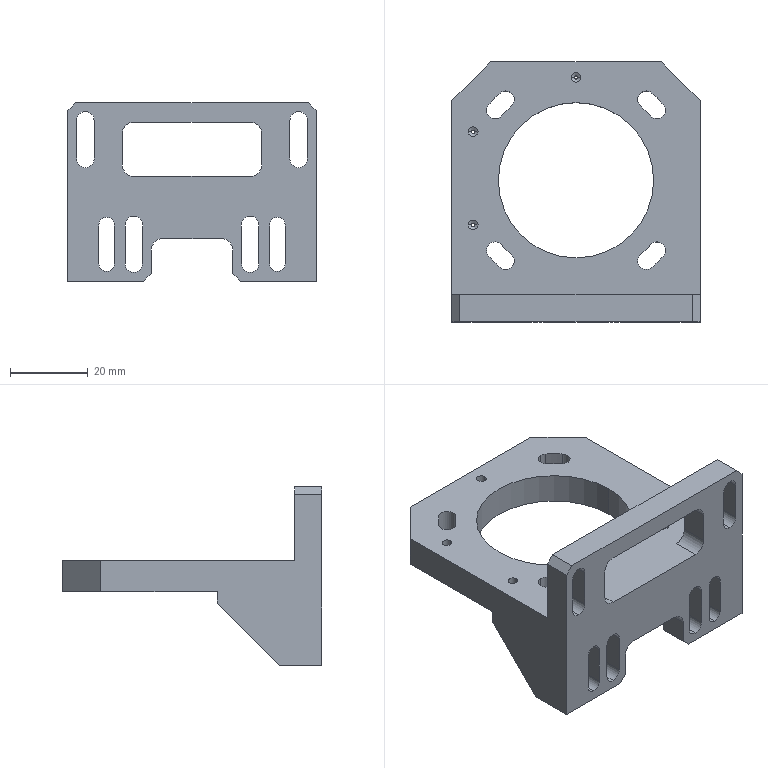NC program | NX | posted with a generic post | part box 64 x 67 x 46 mm
Lines 509 to 1439 of 8734:
(ZLEVEL_PROFILE_COPY_2_COPY , TOOL : D6JING)
N1016 T06 M6
N1018 G54
N1020 G17 G0 G90 X-13.8 Y-11.744 B0. C0. S5000 M3
N1022 G43 Z30. H6
N1024 Z-0.1
N1026 G94 G1 X-14.7 Y-12.264 F1000.
N1028 G3 X-15. Y-12.784 R0.6
N1030 G1 Y-15. F1500.
N1032 X-12.784
N1034 G3 X-12.264 Y-14.7 R0.6
N1036 G1 X-11.744 Y-13.8
N1038 G0 X-13.8 Y-11.744 Z-0.2
N1040 G1 X-14.7 Y-12.264 F1000.
N1042 G3 X-15. Y-12.784 R0.6
N1044 G1 Y-15. F1500.
N1046 X-12.784
N1048 G3 X-12.264 Y-14.7 R0.6
N1050 G1 X-11.744 Y-13.8
N1052 G0 X-13.8 Y-11.744 Z-0.3
N1054 G1 X-14.7 Y-12.264 F1000.
N1056 G3 X-15. Y-12.784 R0.6
N1058 G1 Y-15. F1500.
N1060 X-12.784
N1062 G3 X-12.264 Y-14.7 R0.6
N1064 G1 X-11.744 Y-13.8
N1066 G0 X-13.8 Y-11.744 Z-0.4
N1068 G1 X-14.7 Y-12.264 F1000.
N1070 G3 X-15. Y-12.784 R0.6
N1072 G1 Y-15. F1500.
N1074 X-12.784
N1076 G3 X-12.264 Y-14.7 R0.6
N1078 G1 X-11.744 Y-13.8
N1080 G0 X-13.8 Y-11.744 Z-0.5
N1082 G1 X-14.7 Y-12.264 F1000.
N1084 G3 X-15. Y-12.784 R0.6
N1086 G1 Y-15. F1500.
N1088 X-12.784
N1090 G3 X-12.264 Y-14.7 R0.6
N1092 G1 X-11.744 Y-13.8
N1094 G0 X-13.8 Y-11.744 Z-0.6
N1096 G1 X-14.7 Y-12.264 F1000.
N1098 G3 X-15. Y-12.784 R0.6
N1100 G1 Y-15. F1500.
N1102 X-12.784
N1104 G3 X-12.264 Y-14.7 R0.6
N1106 G1 X-11.744 Y-13.8
N1108 G0 X-13.8 Y-11.744 Z-0.7
N1110 G1 X-14.7 Y-12.264 F1000.
N1112 G3 X-15. Y-12.784 R0.6
N1114 G1 Y-15. F1500.
N1116 X-12.784
N1118 G3 X-12.264 Y-14.7 R0.6
N1120 G1 X-11.744 Y-13.8
N1122 G0 X-13.8 Y-11.744 Z-0.8
N1124 G1 X-14.7 Y-12.264 F1000.
N1126 G3 X-15. Y-12.784 R0.6
N1128 G1 Y-15. F1500.
N1130 X-12.784
N1132 G3 X-12.264 Y-14.7 R0.6
N1134 G1 X-11.744 Y-13.8
N1136 G0 X-13.8 Y-11.744 Z-0.9
N1138 G1 X-14.7 Y-12.264 F1000.
N1140 G3 X-15. Y-12.784 R0.6
N1142 G1 Y-15. F1500.
N1144 X-12.784
N1146 G3 X-12.264 Y-14.7 R0.6
N1148 G1 X-11.744 Y-13.8
N1150 G0 X-13.8 Y-11.744 Z-1.
N1152 G1 X-14.7 Y-12.264 F1000.
N1154 G3 X-15. Y-12.784 R0.6
N1156 G1 Y-15. F1500.
N1158 X-12.784
N1160 G3 X-12.264 Y-14.7 R0.6
N1162 G1 X-11.744 Y-13.8
N1164 G0 X-13.8 Y-11.744 Z-1.1
N1166 G1 X-14.7 Y-12.264 F1000.
N1168 G3 X-15. Y-12.784 R0.6
N1170 G1 Y-15. F1500.
N1172 X-12.784
N1174 G3 X-12.264 Y-14.7 R0.6
N1176 G1 X-11.744 Y-13.8
N1178 G0 X-13.8 Y-11.744 Z-1.2
N1180 G1 X-14.7 Y-12.264 F1000.
N1182 G3 X-15. Y-12.784 R0.6
N1184 G1 Y-15. F1500.
N1186 X-12.784
N1188 G3 X-12.264 Y-14.7 R0.6
N1190 G1 X-11.744 Y-13.8
N1192 G0 X-13.8 Y-11.744 Z-1.3
N1194 G1 X-14.7 Y-12.264 F1000.
N1196 G3 X-15. Y-12.784 R0.6
N1198 G1 Y-15. F1500.
N1200 X-12.784
N1202 G3 X-12.264 Y-14.7 R0.6
N1204 G1 X-11.744 Y-13.8
N1206 G0 X-13.8 Y-11.744 Z-1.4
N1208 G1 X-14.7 Y-12.264 F1000.
N1210 G3 X-15. Y-12.784 R0.6
N1212 G1 Y-15. F1500.
N1214 X-12.784
N1216 G3 X-12.264 Y-14.7 R0.6
N1218 G1 X-11.744 Y-13.8
N1220 G0 X-13.8 Y-11.744 Z-1.5
N1222 G1 X-14.7 Y-12.264 F1000.
N1224 G3 X-15. Y-12.784 R0.6
N1226 G1 Y-15. F1500.
N1228 X-12.784
N1230 G3 X-12.264 Y-14.7 R0.6
N1232 G1 X-11.744 Y-13.8
N1234 G0 X-13.8 Y-11.744 Z-1.6
N1236 G1 X-14.7 Y-12.264 F1000.
N1238 G3 X-15. Y-12.784 R0.6
N1240 G1 Y-15. F1500.
N1242 X-12.784
N1244 G3 X-12.264 Y-14.7 R0.6
N1246 G1 X-11.744 Y-13.8
N1248 G0 X-13.8 Y-11.744 Z-1.7
N1250 G1 X-14.7 Y-12.264 F1000.
N1252 G3 X-15. Y-12.784 R0.6
N1254 G1 Y-15. F1500.
N1256 X-12.784
N1258 G3 X-12.264 Y-14.7 R0.6
N1260 G1 X-11.744 Y-13.8
N1262 G0 X-13.8 Y-11.744 Z-1.8
N1264 G1 X-14.7 Y-12.264 F1000.
N1266 G3 X-15. Y-12.784 R0.6
N1268 G1 Y-15. F1500.
N1270 X-12.784
N1272 G3 X-12.264 Y-14.7 R0.6
N1274 G1 X-11.744 Y-13.8
N1276 G0 X-13.8 Y-11.744 Z-1.9
N1278 G1 X-14.7 Y-12.264 F1000.
N1280 G3 X-15. Y-12.784 R0.6
N1282 G1 Y-15. F1500.
N1284 X-12.784
N1286 G3 X-12.264 Y-14.7 R0.6
N1288 G1 X-11.744 Y-13.8
N1290 G0 X-13.8 Y-11.744 Z-2.
N1292 G1 X-14.7 Y-12.264 F1000.
N1294 G3 X-15. Y-12.784 R0.6
N1296 G1 Y-15. F1500.
N1298 X-12.784
N1300 G3 X-12.264 Y-14.7 R0.6
N1302 G1 X-11.744 Y-13.8
N1304 G0 X-13.8 Y-11.744 Z-2.1
N1306 G1 X-14.7 Y-12.264 F1000.
N1308 G3 X-15. Y-12.784 R0.6
N1310 G1 Y-15. F1500.
N1312 X-12.784
N1314 G3 X-12.264 Y-14.7 R0.6
N1316 G1 X-11.744 Y-13.8
N1318 G0 X-13.8 Y-11.744 Z-2.2
N1320 G1 X-14.7 Y-12.264 F1000.
N1322 G3 X-15. Y-12.784 R0.6
N1324 G1 Y-15. F1500.
N1326 X-12.784
N1328 G3 X-12.264 Y-14.7 R0.6
N1330 G1 X-11.744 Y-13.8
N1332 G0 X-13.8 Y-11.744 Z-2.3
N1334 G1 X-14.7 Y-12.264 F1000.
N1336 G3 X-15. Y-12.784 R0.6
N1338 G1 Y-15. F1500.
N1340 X-12.784
N1342 G3 X-12.264 Y-14.7 R0.6
N1344 G1 X-11.744 Y-13.8
N1346 G0 X-13.8 Y-11.744 Z-2.4
N1348 G1 X-14.7 Y-12.264 F1000.
N1350 G3 X-15. Y-12.784 R0.6
N1352 G1 Y-15. F1500.
N1354 X-12.784
N1356 G3 X-12.264 Y-14.7 R0.6
N1358 G1 X-11.744 Y-13.8
N1360 G0 X-13.8 Y-11.744 Z-2.5
N1362 G1 X-14.7 Y-12.264 F1000.
N1364 G3 X-15. Y-12.784 R0.6
N1366 G1 Y-15. F1500.
N1368 X-12.784
N1370 G3 X-12.264 Y-14.7 R0.6
N1372 G1 X-11.744 Y-13.8
N1374 G0 X-13.8 Y-11.744 Z-2.6
N1376 G1 X-14.7 Y-12.264 F1000.
N1378 G3 X-15. Y-12.784 R0.6
N1380 G1 Y-15. F1500.
N1382 X-12.784
N1384 G3 X-12.264 Y-14.7 R0.6
N1386 G1 X-11.744 Y-13.8
N1388 G0 X-13.8 Y-11.744 Z-2.7
N1390 G1 X-14.7 Y-12.264 F1000.
N1392 G3 X-15. Y-12.784 R0.6
N1394 G1 Y-15. F1500.
N1396 X-12.784
N1398 G3 X-12.264 Y-14.7 R0.6
N1400 G1 X-11.744 Y-13.8
N1402 G0 X-13.8 Y-11.744 Z-2.8
N1404 G1 X-14.7 Y-12.264 F1000.
N1406 G3 X-15. Y-12.784 R0.6
N1408 G1 Y-15. F1500.
N1410 X-12.784
N1412 G3 X-12.264 Y-14.7 R0.6
N1414 G1 X-11.744 Y-13.8
N1416 G0 X-13.8 Y-11.744 Z-2.9
N1418 G1 X-14.7 Y-12.264 F1000.
N1420 G3 X-15. Y-12.784 R0.6
N1422 G1 Y-15. F1500.
N1424 X-12.784
N1426 G3 X-12.264 Y-14.7 R0.6
N1428 G1 X-11.744 Y-13.8
N1430 G0 X-13.8 Y-11.744 Z-3.
N1432 G1 X-14.7 Y-12.264 F1000.
N1434 G3 X-15. Y-12.784 R0.6
N1436 G1 Y-15. F1500.
N1438 X-12.784
N1440 G3 X-12.264 Y-14.7 R0.6
N1442 G1 X-11.744 Y-13.8
N1444 G0 X-13.8 Y-11.744 Z-3.1
N1446 G1 X-14.7 Y-12.264 F1000.
N1448 G3 X-15. Y-12.784 R0.6
N1450 G1 Y-15. F1500.
N1452 X-12.784
N1454 G3 X-12.264 Y-14.7 R0.6
N1456 G1 X-11.744 Y-13.8
N1458 G0 X-13.8 Y-11.744 Z-3.2
N1460 G1 X-14.7 Y-12.264 F1000.
N1462 G3 X-15. Y-12.784 R0.6
N1464 G1 Y-15. F1500.
N1466 X-12.784
N1468 G3 X-12.264 Y-14.7 R0.6
N1470 G1 X-11.744 Y-13.8
N1472 G0 X-13.8 Y-11.744 Z-3.3
N1474 G1 X-14.7 Y-12.264 F1000.
N1476 G3 X-15. Y-12.784 R0.6
N1478 G1 Y-15. F1500.
N1480 X-12.784
N1482 G3 X-12.264 Y-14.7 R0.6
N1484 G1 X-11.744 Y-13.8
N1486 G0 X-13.8 Y-11.744 Z-3.4
N1488 G1 X-14.7 Y-12.264 F1000.
N1490 G3 X-15. Y-12.784 R0.6
N1492 G1 Y-15. F1500.
N1494 X-12.784
N1496 G3 X-12.264 Y-14.7 R0.6
N1498 G1 X-11.744 Y-13.8
N1500 G0 X-13.8 Y-11.744 Z-3.5
N1502 G1 X-14.7 Y-12.264 F1000.
N1504 G3 X-15. Y-12.784 R0.6
N1506 G1 Y-15. F1500.
N1508 X-12.784
N1510 G3 X-12.264 Y-14.7 R0.6
N1512 G1 X-11.744 Y-13.8
N1514 G0 X-13.8 Y-11.744 Z-3.6
N1516 G1 X-14.7 Y-12.264 F1000.
N1518 G3 X-15. Y-12.784 R0.6
N1520 G1 Y-15. F1500.
N1522 X-12.784
N1524 G3 X-12.264 Y-14.7 R0.6
N1526 G1 X-11.744 Y-13.8
N1528 G0 X-13.8 Y-11.744 Z-3.7
N1530 G1 X-14.7 Y-12.264 F1000.
N1532 G3 X-15. Y-12.784 R0.6
N1534 G1 Y-15. F1500.
N1536 X-12.784
N1538 G3 X-12.264 Y-14.7 R0.6
N1540 G1 X-11.744 Y-13.8
N1542 G0 X-13.8 Y-11.744 Z-3.8
N1544 G1 X-14.7 Y-12.264 F1000.
N1546 G3 X-15. Y-12.784 R0.6
N1548 G1 Y-15. F1500.
N1550 X-12.784
N1552 G3 X-12.264 Y-14.7 R0.6
N1554 G1 X-11.744 Y-13.8
N1556 G0 X-13.8 Y-11.744 Z-3.9
N1558 G1 X-14.7 Y-12.264 F1000.
N1560 G3 X-15. Y-12.784 R0.6
N1562 G1 Y-15. F1500.
N1564 X-12.784
N1566 G3 X-12.264 Y-14.7 R0.6
N1568 G1 X-11.744 Y-13.8
N1570 G0 X-13.8 Y-11.744 Z-4.
N1572 G1 X-14.7 Y-12.264 F1000.
N1574 G3 X-15. Y-12.784 R0.6
N1576 G1 Y-15. F1500.
N1578 X-12.784
N1580 G3 X-12.264 Y-14.7 R0.6
N1582 G1 X-11.744 Y-13.8
N1584 G0 X-13.8 Y-11.744 Z-4.1
N1586 G1 X-14.7 Y-12.264 F1000.
N1588 G3 X-15. Y-12.784 R0.6
N1590 G1 Y-15. F1500.
N1592 X-12.784
N1594 G3 X-12.264 Y-14.7 R0.6
N1596 G1 X-11.744 Y-13.8
N1598 G0 X-13.8 Y-11.744 Z-4.2
N1600 G1 X-14.7 Y-12.264 F1000.
N1602 G3 X-15. Y-12.784 R0.6
N1604 G1 Y-15. F1500.
N1606 X-12.784
N1608 G3 X-12.264 Y-14.7 R0.6
N1610 G1 X-11.744 Y-13.8
N1612 G0 X-13.8 Y-11.744 Z-4.3
N1614 G1 X-14.7 Y-12.264 F1000.
N1616 G3 X-15. Y-12.784 R0.6
N1618 G1 Y-15. F1500.
N1620 X-12.784
N1622 G3 X-12.264 Y-14.7 R0.6
N1624 G1 X-11.744 Y-13.8
N1626 G0 X-13.8 Y-11.744 Z-4.4
N1628 G1 X-14.7 Y-12.264 F1000.
N1630 G3 X-15. Y-12.784 R0.6
N1632 G1 Y-15. F1500.
N1634 X-12.784
N1636 G3 X-12.264 Y-14.7 R0.6
N1638 G1 X-11.744 Y-13.8
N1640 G0 X-13.8 Y-11.744 Z-4.5
N1642 G1 X-14.7 Y-12.264 F1000.
N1644 G3 X-15. Y-12.784 R0.6
N1646 G1 Y-15. F1500.
N1648 X-12.784
N1650 G3 X-12.264 Y-14.7 R0.6
N1652 G1 X-11.744 Y-13.8
N1654 G0 X-13.8 Y-11.744 Z-4.6
N1656 G1 X-14.7 Y-12.264 F1000.
N1658 G3 X-15. Y-12.784 R0.6
N1660 G1 Y-15. F1500.
N1662 X-12.784
N1664 G3 X-12.264 Y-14.7 R0.6
N1666 G1 X-11.744 Y-13.8
N1668 G0 X-13.8 Y-11.744 Z-4.7
N1670 G1 X-14.7 Y-12.264 F1000.
N1672 G3 X-15. Y-12.784 R0.6
N1674 G1 Y-15. F1500.
N1676 X-12.784
N1678 G3 X-12.264 Y-14.7 R0.6
N1680 G1 X-11.744 Y-13.8
N1682 G0 X-13.8 Y-11.744 Z-4.8
N1684 G1 X-14.7 Y-12.264 F1000.
N1686 G3 X-15. Y-12.784 R0.6
N1688 G1 Y-15. F1500.
N1690 X-12.784
N1692 G3 X-12.264 Y-14.7 R0.6
N1694 G1 X-11.744 Y-13.8
N1696 G0 X-13.8 Y-11.744 Z-4.9
N1698 G1 X-14.7 Y-12.264 F1000.
N1700 G3 X-15. Y-12.784 R0.6
N1702 G1 Y-15. F1500.
N1704 X-12.784
N1706 G3 X-12.264 Y-14.7 R0.6
N1708 G1 X-11.744 Y-13.8
N1710 G0 X-13.8 Y-11.744 Z-5.
N1712 G1 X-14.7 Y-12.264 F1000.
N1714 G3 X-15. Y-12.784 R0.6
N1716 G1 Y-15. F1500.
N1718 X-12.784
N1720 G3 X-12.264 Y-14.7 R0.6
N1722 G1 X-11.744 Y-13.8
N1724 G0 X-13.8 Y-11.744 Z-5.1
N1726 G1 X-14.7 Y-12.264 F1000.
N1728 G3 X-15. Y-12.784 R0.6
N1730 G1 Y-15. F1500.
N1732 X-12.784
N1734 G3 X-12.264 Y-14.7 R0.6
N1736 G1 X-11.744 Y-13.8
N1738 G0 X-13.8 Y-11.744 Z-5.2
N1740 G1 X-14.7 Y-12.264 F1000.
N1742 G3 X-15. Y-12.784 R0.6
N1744 G1 Y-15. F1500.
N1746 X-12.784
N1748 G3 X-12.264 Y-14.7 R0.6
N1750 G1 X-11.744 Y-13.8
N1752 G0 X-13.8 Y-11.744 Z-5.3
N1754 G1 X-14.7 Y-12.264 F1000.
N1756 G3 X-15. Y-12.784 R0.6
N1758 G1 Y-15. F1500.
N1760 X-12.784
N1762 G3 X-12.264 Y-14.7 R0.6
N1764 G1 X-11.744 Y-13.8
N1766 G0 X-13.8 Y-11.744 Z-5.4
N1768 G1 X-14.7 Y-12.264 F1000.
N1770 G3 X-15. Y-12.784 R0.6
N1772 G1 Y-15. F1500.
N1774 X-12.784
N1776 G3 X-12.264 Y-14.7 R0.6
N1778 G1 X-11.744 Y-13.8
N1780 G0 X-13.8 Y-11.744 Z-5.5
N1782 G1 X-14.7 Y-12.264 F1000.
N1784 G3 X-15. Y-12.784 R0.6
N1786 G1 Y-15. F1500.
N1788 X-12.784
N1790 G3 X-12.264 Y-14.7 R0.6
N1792 G1 X-11.744 Y-13.8
N1794 G0 X-13.8 Y-11.744 Z-5.6
N1796 G1 X-14.7 Y-12.264 F1000.
N1798 G3 X-15. Y-12.784 R0.6
N1800 G1 Y-15. F1500.
N1802 X-12.784
N1804 G3 X-12.264 Y-14.7 R0.6
N1806 G1 X-11.744 Y-13.8
N1808 G0 X-13.8 Y-11.744 Z-5.7
N1810 G1 X-14.7 Y-12.264 F1000.
N1812 G3 X-15. Y-12.784 R0.6
N1814 G1 Y-15. F1500.
N1816 X-12.784
N1818 G3 X-12.264 Y-14.7 R0.6
N1820 G1 X-11.744 Y-13.8
N1822 G0 X-13.8 Y-11.744 Z-5.8
N1824 G1 X-14.7 Y-12.264 F1000.
N1826 G3 X-15. Y-12.784 R0.6
N1828 G1 Y-15. F1500.
N1830 X-12.784
N1832 G3 X-12.264 Y-14.7 R0.6
N1834 G1 X-11.744 Y-13.8
N1836 G0 X-13.8 Y-11.744 Z-5.9
N1838 G1 X-14.7 Y-12.264 F1000.
N1840 G3 X-15. Y-12.784 R0.6
N1842 G1 Y-15. F1500.
N1844 X-12.784
N1846 G3 X-12.264 Y-14.7 R0.6
N1848 G1 X-11.744 Y-13.8
N1850 G0 X-13.8 Y-11.744 Z-6.
N1852 G1 X-14.7 Y-12.264 F1000.
N1854 G3 X-15. Y-12.784 R0.6
N1856 G1 Y-15. F1500.
N1858 X-12.784
N1860 G3 X-12.264 Y-14.7 R0.6
N1862 G1 X-11.744 Y-13.8
N1864 G0 X-13.8 Y-11.744 Z-6.1
N1866 G1 X-14.7 Y-12.264 F1000.
N1868 G3 X-15. Y-12.784 R0.6
N1870 G1 Y-15. F1500.
N1872 X-12.784
N1874 G3 X-12.264 Y-14.7 R0.6
N1876 G1 X-11.744 Y-13.8
N1878 G0 X-13.8 Y-11.744 Z-6.2
N1880 G1 X-14.7 Y-12.264 F1000.
N1882 G3 X-15. Y-12.784 R0.6
N1884 G1 Y-15. F1500.
N1886 X-12.784
N1888 G3 X-12.264 Y-14.7 R0.6
N1890 G1 X-11.744 Y-13.8
N1892 G0 X-13.8 Y-11.744 Z-6.3
N1894 G1 X-14.7 Y-12.264 F1000.
N1896 G3 X-15. Y-12.784 R0.6
N1898 G1 Y-15. F1500.
N1900 X-12.784
N1902 G3 X-12.264 Y-14.7 R0.6
N1904 G1 X-11.744 Y-13.8
N1906 G0 X-13.8 Y-11.744 Z-6.4
N1908 G1 X-14.7 Y-12.264 F1000.
N1910 G3 X-15. Y-12.784 R0.6
N1912 G1 Y-15. F1500.
N1914 X-12.784
N1916 G3 X-12.264 Y-14.7 R0.6
N1918 G1 X-11.744 Y-13.8
N1920 G0 X-13.8 Y-11.744 Z-6.5
N1922 G1 X-14.7 Y-12.264 F1000.
N1924 G3 X-15. Y-12.784 R0.6
N1926 G1 Y-15. F1500.
N1928 X-12.784
N1930 G3 X-12.264 Y-14.7 R0.6
N1932 G1 X-11.744 Y-13.8
N1934 G0 X-13.8 Y-11.744 Z-6.6
N1936 G1 X-14.7 Y-12.264 F1000.
N1938 G3 X-15. Y-12.784 R0.6
N1940 G1 Y-15. F1500.
N1942 X-12.784
N1944 G3 X-12.264 Y-14.7 R0.6
N1946 G1 X-11.744 Y-13.8
N1948 G0 X-13.8 Y-11.744 Z-6.7
N1950 G1 X-14.7 Y-12.264 F1000.
N1952 G3 X-15. Y-12.784 R0.6
N1954 G1 Y-15. F1500.
N1956 X-12.784
N1958 G3 X-12.264 Y-14.7 R0.6
N1960 G1 X-11.744 Y-13.8
N1962 G0 X-13.8 Y-11.744 Z-6.8
N1964 G1 X-14.7 Y-12.264 F1000.
N1966 G3 X-15. Y-12.784 R0.6
N1968 G1 Y-15. F1500.
N1970 X-12.784
N1972 G3 X-12.264 Y-14.7 R0.6
N1974 G1 X-11.744 Y-13.8
N1976 G0 X-13.8 Y-11.744 Z-6.9
N1978 G1 X-14.7 Y-12.264 F1000.
N1980 G3 X-15. Y-12.784 R0.6
N1982 G1 Y-15. F1500.
N1984 X-12.784
N1986 G3 X-12.264 Y-14.7 R0.6
N1988 G1 X-11.744 Y-13.8
N1990 G0 X-13.8 Y-11.744 Z-7.
N1992 G1 X-14.7 Y-12.264 F1000.
N1994 G3 X-15. Y-12.784 R0.6
N1996 G1 Y-15. F1500.
N1998 X-12.784
N2000 G3 X-12.264 Y-14.7 R0.6
N2002 G1 X-11.744 Y-13.8
N2004 G0 Z30.
N2006 X11.744
N2008 Z-0.1
N2010 G1 X12.264 Y-14.7 F1000.
N2012 G3 X12.784 Y-15. R0.6
N2014 G1 X15. F1500.
N2016 Y-12.784
N2018 G3 X14.7 Y-12.264 R0.6
N2020 G1 X13.8 Y-11.744
N2022 G0 X11.744 Y-13.8 Z-0.2
N2024 G1 X12.264 Y-14.7 F1000.
N2026 G3 X12.784 Y-15. R0.6
N2028 G1 X15. F1500.
N2030 Y-12.784
N2032 G3 X14.7 Y-12.264 R0.6
N2034 G1 X13.8 Y-11.744
N2036 G0 X11.744 Y-13.8 Z-0.3
N2038 G1 X12.264 Y-14.7 F1000.
N2040 G3 X12.784 Y-15. R0.6
N2042 G1 X15. F1500.
N2044 Y-12.784
N2046 G3 X14.7 Y-12.264 R0.6
N2048 G1 X13.8 Y-11.744
N2050 G0 X11.744 Y-13.8 Z-0.4
N2052 G1 X12.264 Y-14.7 F1000.
N2054 G3 X12.784 Y-15. R0.6
N2056 G1 X15. F1500.
N2058 Y-12.784
N2060 G3 X14.7 Y-12.264 R0.6
N2062 G1 X13.8 Y-11.744
N2064 G0 X11.744 Y-13.8 Z-0.5
N2066 G1 X12.264 Y-14.7 F1000.
N2068 G3 X12.784 Y-15. R0.6
N2070 G1 X15. F1500.
N2072 Y-12.784
N2074 G3 X14.7 Y-12.264 R0.6
N2076 G1 X13.8 Y-11.744
N2078 G0 X11.744 Y-13.8 Z-0.6
N2080 G1 X12.264 Y-14.7 F1000.
N2082 G3 X12.784 Y-15. R0.6
N2084 G1 X15. F1500.
N2086 Y-12.784
N2088 G3 X14.7 Y-12.264 R0.6
N2090 G1 X13.8 Y-11.744
N2092 G0 X11.744 Y-13.8 Z-0.7
N2094 G1 X12.264 Y-14.7 F1000.
N2096 G3 X12.784 Y-15. R0.6
N2098 G1 X15. F1500.
N2100 Y-12.784
N2102 G3 X14.7 Y-12.264 R0.6
N2104 G1 X13.8 Y-11.744
N2106 G0 X11.744 Y-13.8 Z-0.8
N2108 G1 X12.264 Y-14.7 F1000.
N2110 G3 X12.784 Y-15. R0.6
N2112 G1 X15. F1500.
N2114 Y-12.784
N2116 G3 X14.7 Y-12.264 R0.6
N2118 G1 X13.8 Y-11.744
N2120 G0 X11.744 Y-13.8 Z-0.9
N2122 G1 X12.264 Y-14.7 F1000.
N2124 G3 X12.784 Y-15. R0.6
N2126 G1 X15. F1500.
N2128 Y-12.784
N2130 G3 X14.7 Y-12.264 R0.6
N2132 G1 X13.8 Y-11.744
N2134 G0 X11.744 Y-13.8 Z-1.
N2136 G1 X12.264 Y-14.7 F1000.
N2138 G3 X12.784 Y-15. R0.6
N2140 G1 X15. F1500.
N2142 Y-12.784
N2144 G3 X14.7 Y-12.264 R0.6
N2146 G1 X13.8 Y-11.744
N2148 G0 X11.744 Y-13.8 Z-1.1
N2150 G1 X12.264 Y-14.7 F1000.
N2152 G3 X12.784 Y-15. R0.6
N2154 G1 X15. F1500.
N2156 Y-12.784
N2158 G3 X14.7 Y-12.264 R0.6
N2160 G1 X13.8 Y-11.744
N2162 G0 X11.744 Y-13.8 Z-1.2
N2164 G1 X12.264 Y-14.7 F1000.
N2166 G3 X12.784 Y-15. R0.6
N2168 G1 X15. F1500.
N2170 Y-12.784
N2172 G3 X14.7 Y-12.264 R0.6
N2174 G1 X13.8 Y-11.744
N2176 G0 X11.744 Y-13.8 Z-1.3
N2178 G1 X12.264 Y-14.7 F1000.
N2180 G3 X12.784 Y-15. R0.6
N2182 G1 X15. F1500.
N2184 Y-12.784
N2186 G3 X14.7 Y-12.264 R0.6
N2188 G1 X13.8 Y-11.744
N2190 G0 X11.744 Y-13.8 Z-1.4
N2192 G1 X12.264 Y-14.7 F1000.
N2194 G3 X12.784 Y-15. R0.6
N2196 G1 X15. F1500.
N2198 Y-12.784
N2200 G3 X14.7 Y-12.264 R0.6
N2202 G1 X13.8 Y-11.744
N2204 G0 X11.744 Y-13.8 Z-1.5
N2206 G1 X12.264 Y-14.7 F1000.
N2208 G3 X12.784 Y-15. R0.6
N2210 G1 X15. F1500.
N2212 Y-12.784
N2214 G3 X14.7 Y-12.264 R0.6
N2216 G1 X13.8 Y-11.744
N2218 G0 X11.744 Y-13.8 Z-1.6
N2220 G1 X12.264 Y-14.7 F1000.
N2222 G3 X12.784 Y-15. R0.6
N2224 G1 X15. F1500.
N2226 Y-12.784
N2228 G3 X14.7 Y-12.264 R0.6
N2230 G1 X13.8 Y-11.744
N2232 G0 X11.744 Y-13.8 Z-1.7
N2234 G1 X12.264 Y-14.7 F1000.
N2236 G3 X12.784 Y-15. R0.6
N2238 G1 X15. F1500.
N2240 Y-12.784
N2242 G3 X14.7 Y-12.264 R0.6
N2244 G1 X13.8 Y-11.744
N2246 G0 X11.744 Y-13.8 Z-1.8
N2248 G1 X12.264 Y-14.7 F1000.
N2250 G3 X12.784 Y-15. R0.6
N2252 G1 X15. F1500.
N2254 Y-12.784
N2256 G3 X14.7 Y-12.264 R0.6
N2258 G1 X13.8 Y-11.744
N2260 G0 X11.744 Y-13.8 Z-1.9
N2262 G1 X12.264 Y-14.7 F1000.
N2264 G3 X12.784 Y-15. R0.6
N2266 G1 X15. F1500.
N2268 Y-12.784
N2270 G3 X14.7 Y-12.264 R0.6
N2272 G1 X13.8 Y-11.744
N2274 G0 X11.744 Y-13.8 Z-2.
N2276 G1 X12.264 Y-14.7 F1000.
N2278 G3 X12.784 Y-15. R0.6
N2280 G1 X15. F1500.
N2282 Y-12.784
N2284 G3 X14.7 Y-12.264 R0.6
N2286 G1 X13.8 Y-11.744
N2288 G0 X11.744 Y-13.8 Z-2.1
N2290 G1 X12.264 Y-14.7 F1000.
N2292 G3 X12.784 Y-15. R0.6
N2294 G1 X15. F1500.
N2296 Y-12.784
N2298 G3 X14.7 Y-12.264 R0.6
N2300 G1 X13.8 Y-11.744
N2302 G0 X11.744 Y-13.8 Z-2.2
N2304 G1 X12.264 Y-14.7 F1000.
N2306 G3 X12.784 Y-15. R0.6
N2308 G1 X15. F1500.
N2310 Y-12.784
N2312 G3 X14.7 Y-12.264 R0.6
N2314 G1 X13.8 Y-11.744
N2316 G0 X11.744 Y-13.8 Z-2.3
N2318 G1 X12.264 Y-14.7 F1000.
N2320 G3 X12.784 Y-15. R0.6
N2322 G1 X15. F1500.
N2324 Y-12.784
N2326 G3 X14.7 Y-12.264 R0.6
N2328 G1 X13.8 Y-11.744
N2330 G0 X11.744 Y-13.8 Z-2.4
N2332 G1 X12.264 Y-14.7 F1000.
N2334 G3 X12.784 Y-15. R0.6
N2336 G1 X15. F1500.
N2338 Y-12.784
N2340 G3 X14.7 Y-12.264 R0.6
N2342 G1 X13.8 Y-11.744
N2344 G0 X11.744 Y-13.8 Z-2.5
N2346 G1 X12.264 Y-14.7 F1000.
N2348 G3 X12.784 Y-15. R0.6
N2350 G1 X15. F1500.
N2352 Y-12.784
N2354 G3 X14.7 Y-12.264 R0.6
N2356 G1 X13.8 Y-11.744
N2358 G0 X11.744 Y-13.8 Z-2.6
N2360 G1 X12.264 Y-14.7 F1000.
N2362 G3 X12.784 Y-15. R0.6
N2364 G1 X15. F1500.
N2366 Y-12.784
N2368 G3 X14.7 Y-12.264 R0.6
N2370 G1 X13.8 Y-11.744
N2372 G0 X11.744 Y-13.8 Z-2.7
N2374 G1 X12.264 Y-14.7 F1000.
N2376 G3 X12.784 Y-15. R0.6
N2378 G1 X15. F1500.
N2380 Y-12.784
N2382 G3 X14.7 Y-12.264 R0.6
N2384 G1 X13.8 Y-11.744
N2386 G0 X11.744 Y-13.8 Z-2.8
N2388 G1 X12.264 Y-14.7 F1000.
N2390 G3 X12.784 Y-15. R0.6
N2392 G1 X15. F1500.
N2394 Y-12.784
N2396 G3 X14.7 Y-12.264 R0.6
N2398 G1 X13.8 Y-11.744
N2400 G0 X11.744 Y-13.8 Z-2.9
N2402 G1 X12.264 Y-14.7 F1000.
N2404 G3 X12.784 Y-15. R0.6
N2406 G1 X15. F1500.
N2408 Y-12.784
N2410 G3 X14.7 Y-12.264 R0.6
N2412 G1 X13.8 Y-11.744
N2414 G0 X11.744 Y-13.8 Z-3.
N2416 G1 X12.264 Y-14.7 F1000.
N2418 G3 X12.784 Y-15. R0.6
N2420 G1 X15. F1500.
N2422 Y-12.784
N2424 G3 X14.7 Y-12.264 R0.6
N2426 G1 X13.8 Y-11.744
N2428 G0 X11.744 Y-13.8 Z-3.1
N2430 G1 X12.264 Y-14.7 F1000.
N2432 G3 X12.784 Y-15. R0.6
N2434 G1 X15. F1500.
N2436 Y-12.784
N2438 G3 X14.7 Y-12.264 R0.6
N2440 G1 X13.8 Y-11.744
N2442 G0 X11.744 Y-13.8 Z-3.2
N2444 G1 X12.264 Y-14.7 F1000.
N2446 G3 X12.784 Y-15. R0.6
N2448 G1 X15. F1500.
N2450 Y-12.784
N2452 G3 X14.7 Y-12.264 R0.6
N2454 G1 X13.8 Y-11.744
N2456 G0 X11.744 Y-13.8 Z-3.3
N2458 G1 X12.264 Y-14.7 F1000.
N2460 G3 X12.784 Y-15. R0.6
N2462 G1 X15. F1500.
N2464 Y-12.784
N2466 G3 X14.7 Y-12.264 R0.6
N2468 G1 X13.8 Y-11.744
N2470 G0 X11.744 Y-13.8 Z-3.4
N2472 G1 X12.264 Y-14.7 F1000.
N2474 G3 X12.784 Y-15. R0.6
N2476 G1 X15. F1500.
N2478 Y-12.784
N2480 G3 X14.7 Y-12.264 R0.6
N2482 G1 X13.8 Y-11.744
N2484 G0 X11.744 Y-13.8 Z-3.5
N2486 G1 X12.264 Y-14.7 F1000.
N2488 G3 X12.784 Y-15. R0.6
N2490 G1 X15. F1500.
N2492 Y-12.784
N2494 G3 X14.7 Y-12.264 R0.6
N2496 G1 X13.8 Y-11.744
N2498 G0 X11.744 Y-13.8 Z-3.6
N2500 G1 X12.264 Y-14.7 F1000.
N2502 G3 X12.784 Y-15. R0.6
N2504 G1 X15. F1500.
N2506 Y-12.784
N2508 G3 X14.7 Y-12.264 R0.6
N2510 G1 X13.8 Y-11.744
N2512 G0 X11.744 Y-13.8 Z-3.7
N2514 G1 X12.264 Y-14.7 F1000.
N2516 G3 X12.784 Y-15. R0.6
N2518 G1 X15. F1500.
N2520 Y-12.784
N2522 G3 X14.7 Y-12.264 R0.6
N2524 G1 X13.8 Y-11.744
N2526 G0 X11.744 Y-13.8 Z-3.8
N2528 G1 X12.264 Y-14.7 F1000.
N2530 G3 X12.784 Y-15. R0.6
N2532 G1 X15. F1500.
N2534 Y-12.784
N2536 G3 X14.7 Y-12.264 R0.6
N2538 G1 X13.8 Y-11.744
N2540 G0 X11.744 Y-13.8 Z-3.9
N2542 G1 X12.264 Y-14.7 F1000.
N2544 G3 X12.784 Y-15. R0.6
N2546 G1 X15. F1500.
N2548 Y-12.784
N2550 G3 X14.7 Y-12.264 R0.6
N2552 G1 X13.8 Y-11.744
N2554 G0 X11.744 Y-13.8 Z-4.
N2556 G1 X12.264 Y-14.7 F1000.
N2558 G3 X12.784 Y-15. R0.6
N2560 G1 X15. F1500.
N2562 Y-12.784
N2564 G3 X14.7 Y-12.264 R0.6
N2566 G1 X13.8 Y-11.744
N2568 G0 X11.744 Y-13.8 Z-4.1
N2570 G1 X12.264 Y-14.7 F1000.
N2572 G3 X12.784 Y-15. R0.6
N2574 G1 X15. F1500.
N2576 Y-12.784
N2578 G3 X14.7 Y-12.264 R0.6
N2580 G1 X13.8 Y-11.744
N2582 G0 X11.744 Y-13.8 Z-4.2
N2584 G1 X12.264 Y-14.7 F1000.
N2586 G3 X12.784 Y-15. R0.6
N2588 G1 X15. F1500.
N2590 Y-12.784
N2592 G3 X14.7 Y-12.264 R0.6
N2594 G1 X13.8 Y-11.744
N2596 G0 X11.744 Y-13.8 Z-4.3
N2598 G1 X12.264 Y-14.7 F1000.
N2600 G3 X12.784 Y-15. R0.6
N2602 G1 X15. F1500.
N2604 Y-12.784
N2606 G3 X14.7 Y-12.264 R0.6
N2608 G1 X13.8 Y-11.744
N2610 G0 X11.744 Y-13.8 Z-4.4
N2612 G1 X12.264 Y-14.7 F1000.
N2614 G3 X12.784 Y-15. R0.6
N2616 G1 X15. F1500.
N2618 Y-12.784
N2620 G3 X14.7 Y-12.264 R0.6
N2622 G1 X13.8 Y-11.744
N2624 G0 X11.744 Y-13.8 Z-4.5
N2626 G1 X12.264 Y-14.7 F1000.
N2628 G3 X12.784 Y-15. R0.6
N2630 G1 X15. F1500.
N2632 Y-12.784
N2634 G3 X14.7 Y-12.264 R0.6
N2636 G1 X13.8 Y-11.744
N2638 G0 X11.744 Y-13.8 Z-4.6
N2640 G1 X12.264 Y-14.7 F1000.
N2642 G3 X12.784 Y-15. R0.6
N2644 G1 X15. F1500.
N2646 Y-12.784
N2648 G3 X14.7 Y-12.264 R0.6
N2650 G1 X13.8 Y-11.744
N2652 G0 X11.744 Y-13.8 Z-4.7
N2654 G1 X12.264 Y-14.7 F1000.
N2656 G3 X12.784 Y-15. R0.6
N2658 G1 X15. F1500.
N2660 Y-12.784
N2662 G3 X14.7 Y-12.264 R0.6
N2664 G1 X13.8 Y-11.744
N2666 G0 X11.744 Y-13.8 Z-4.8
N2668 G1 X12.264 Y-14.7 F1000.
N2670 G3 X12.784 Y-15. R0.6
N2672 G1 X15. F1500.
N2674 Y-12.784
N2676 G3 X14.7 Y-12.264 R0.6
N2678 G1 X13.8 Y-11.744
N2680 G0 X11.744 Y-13.8 Z-4.9
N2682 G1 X12.264 Y-14.7 F1000.
N2684 G3 X12.784 Y-15. R0.6
N2686 G1 X15. F1500.
N2688 Y-12.784
N2690 G3 X14.7 Y-12.264 R0.6
N2692 G1 X13.8 Y-11.744
N2694 G0 X11.744 Y-13.8 Z-5.
N2696 G1 X12.264 Y-14.7 F1000.
N2698 G3 X12.784 Y-15. R0.6
N2700 G1 X15. F1500.
N2702 Y-12.784
N2704 G3 X14.7 Y-12.264 R0.6
N2706 G1 X13.8 Y-11.744
N2708 G0 X11.744 Y-13.8 Z-5.1
N2710 G1 X12.264 Y-14.7 F1000.
N2712 G3 X12.784 Y-15. R0.6
N2714 G1 X15. F1500.
N2716 Y-12.784
N2718 G3 X14.7 Y-12.264 R0.6
N2720 G1 X13.8 Y-11.744
N2722 G0 X11.744 Y-13.8 Z-5.2
N2724 G1 X12.264 Y-14.7 F1000.
N2726 G3 X12.784 Y-15. R0.6
N2728 G1 X15. F1500.
N2730 Y-12.784
N2732 G3 X14.7 Y-12.264 R0.6
N2734 G1 X13.8 Y-11.744
N2736 G0 X11.744 Y-13.8 Z-5.3
N2738 G1 X12.264 Y-14.7 F1000.
N2740 G3 X12.784 Y-15. R0.6
N2742 G1 X15. F1500.
N2744 Y-12.784
N2746 G3 X14.7 Y-12.264 R0.6
N2748 G1 X13.8 Y-11.744
N2750 G0 X11.744 Y-13.8 Z-5.4
N2752 G1 X12.264 Y-14.7 F1000.
N2754 G3 X12.784 Y-15. R0.6
N2756 G1 X15. F1500.
N2758 Y-12.784
N2760 G3 X14.7 Y-12.264 R0.6
N2762 G1 X13.8 Y-11.744
N2764 G0 X11.744 Y-13.8 Z-5.5
N2766 G1 X12.264 Y-14.7 F1000.
N2768 G3 X12.784 Y-15. R0.6
N2770 G1 X15. F1500.
N2772 Y-12.784
N2774 G3 X14.7 Y-12.264 R0.6
N2776 G1 X13.8 Y-11.744
N2778 G0 X11.744 Y-13.8 Z-5.6
N2780 G1 X12.264 Y-14.7 F1000.
N2782 G3 X12.784 Y-15. R0.6
N2784 G1 X15. F1500.
N2786 Y-12.784
N2788 G3 X14.7 Y-12.264 R0.6
N2790 G1 X13.8 Y-11.744
N2792 G0 X11.744 Y-13.8 Z-5.7
N2794 G1 X12.264 Y-14.7 F1000.
N2796 G3 X12.784 Y-15. R0.6
N2798 G1 X15. F1500.
N2800 Y-12.784
N2802 G3 X14.7 Y-12.264 R0.6
N2804 G1 X13.8 Y-11.744
N2806 G0 X11.744 Y-13.8 Z-5.8
N2808 G1 X12.264 Y-14.7 F1000.
N2810 G3 X12.784 Y-15. R0.6
N2812 G1 X15. F1500.
N2814 Y-12.784
N2816 G3 X14.7 Y-12.264 R0.6
N2818 G1 X13.8 Y-11.744
N2820 G0 X11.744 Y-13.8 Z-5.9
N2822 G1 X12.264 Y-14.7 F1000.
N2824 G3 X12.784 Y-15. R0.6
N2826 G1 X15. F1500.
N2828 Y-12.784
N2830 G3 X14.7 Y-12.264 R0.6
N2832 G1 X13.8 Y-11.744
N2834 G0 X11.744 Y-13.8 Z-6.
N2836 G1 X12.264 Y-14.7 F1000.
N2838 G3 X12.784 Y-15. R0.6
N2840 G1 X15. F1500.
N2842 Y-12.784
N2844 G3 X14.7 Y-12.264 R0.6
N2846 G1 X13.8 Y-11.744
N2848 G0 X11.744 Y-13.8 Z-6.1
N2850 G1 X12.264 Y-14.7 F1000.
N2852 G3 X12.784 Y-15. R0.6
N2854 G1 X15. F1500.
N2856 Y-12.784
N2858 G3 X14.7 Y-12.264 R0.6
N2860 G1 X13.8 Y-11.744
N2862 G0 X11.744 Y-13.8 Z-6.2
N2864 G1 X12.264 Y-14.7 F1000.
N2866 G3 X12.784 Y-15. R0.6
N2868 G1 X15. F1500.
N2870 Y-12.784